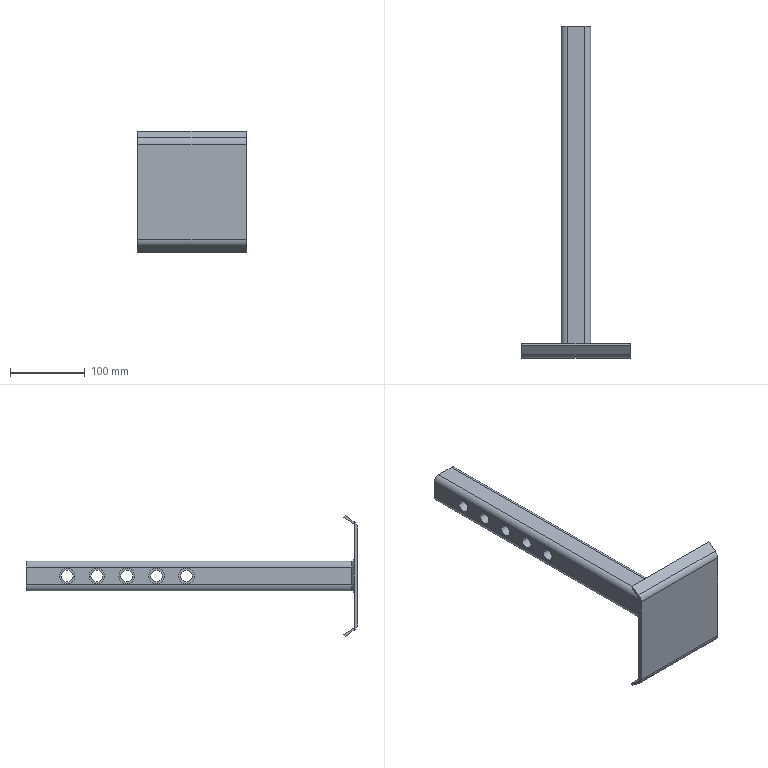Part | STEP file | STOPA_KOMBAJNV11_Default<Obrobiona> | 11 solids | 113 faces | box 145 x 445 x 162.836 mm | volume 371742 mm3 | cylinder 58 | plane 51 | cone 4 | commonest cylinder face diameters 21 x30 16 x18 8 x8 20 x2